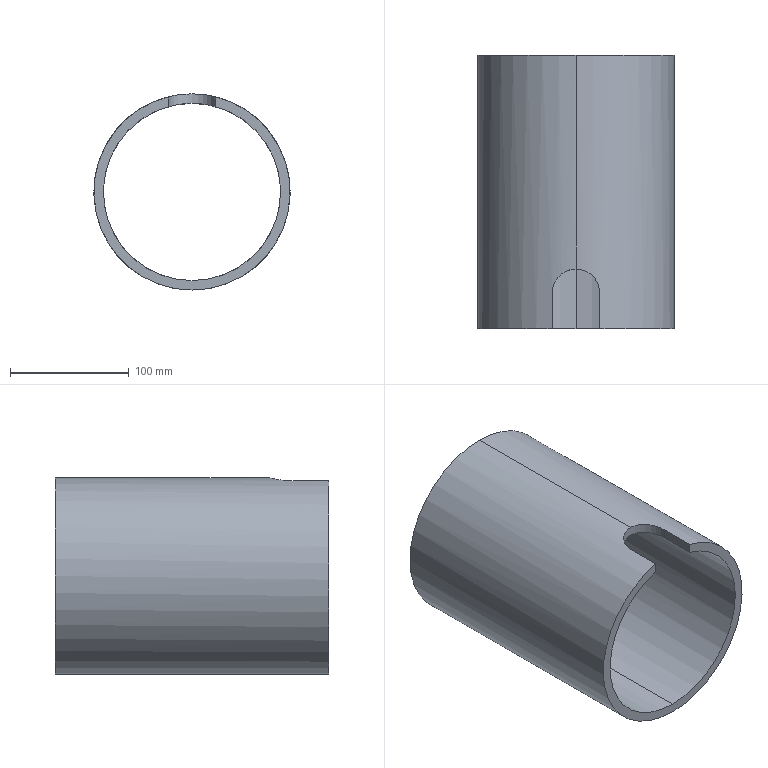Part | SolidWorks | features Extrusion 1, ICE 1 | 1 solid | 9 faces | box 165 x 230 x 165 mm | volume 892768 mm3 | cylinder 5 | plane 4 | commonest cylinder face diameters 149 x2 165 x2 40 x1
STEP:
#1=CARTESIAN_POINT('',(0.,230.,-74.5));
#2=VERTEX_POINT('',#1);
#3=CARTESIAN_POINT('',(0.,230.,74.5));
#4=VERTEX_POINT('',#3);
#5=CARTESIAN_POINT('',(0.,230.,0.));
#6=DIRECTION('',(0.,1.,0.));
#7=DIRECTION('',(0.,0.,1.));
#8=AXIS2_PLACEMENT_3D('',#5,#6,#7);
#9=CIRCLE('',#8,74.5);
#10=EDGE_CURVE('',#2,#4,#9,.T.);
#11=ORIENTED_EDGE('',*,*,#10,.T.);
#12=CARTESIAN_POINT('',(0.,50.,74.5));
#13=VERTEX_POINT('',#12);
#14=CARTESIAN_POINT('',(0.,230.,74.5));
#15=DIRECTION('',(0.,-1.,0.));
#16=VECTOR('',#15,1000.);
#17=LINE('',#14,#16);
#18=EDGE_CURVE('',#4,#13,#17,.T.);
#19=ORIENTED_EDGE('',*,*,#18,.T.);
#20=CARTESIAN_POINT('',(-20.,30.,71.765));
#21=VERTEX_POINT('',#20);
#22=CARTESIAN_POINT('',(-20.,30.,71.765));
#23=CARTESIAN_POINT('',(-20.,31.328,71.765));
#24=CARTESIAN_POINT('',(-19.869,32.633,71.802));
#25=CARTESIAN_POINT('',(-19.485,34.557,71.907));
#26=CARTESIAN_POINT('',(-19.325,35.193,71.95));
#27=CARTESIAN_POINT('',(-18.942,36.453,72.052));
#28=CARTESIAN_POINT('',(-18.717,37.077,72.111));
#29=CARTESIAN_POINT('',(-17.962,38.892,72.304));
#30=CARTESIAN_POINT('',(-17.347,40.038,72.456));
#31=CARTESIAN_POINT('',(-16.258,41.666,72.705));
#32=CARTESIAN_POINT('',(-15.865,42.195,72.792));
#33=CARTESIAN_POINT('',(-15.033,43.207,72.969));
#34=CARTESIAN_POINT('',(-14.595,43.689,73.058));
#35=CARTESIAN_POINT('',(-13.218,45.066,73.324));
#36=CARTESIAN_POINT('',(-12.214,45.892,73.5));
#37=CARTESIAN_POINT('',(-10.575,46.989,73.748));
#38=CARTESIAN_POINT('',(-10.011,47.327,73.827));
#39=CARTESIAN_POINT('',(-8.86,47.942,73.974));
#40=CARTESIAN_POINT('',(-8.272,48.221,74.042));
#41=CARTESIAN_POINT('',(-7.069,48.72,74.166));
#42=CARTESIAN_POINT('',(-6.455,48.941,74.223));
#43=CARTESIAN_POINT('',(-5.199,49.324,74.321));
#44=CARTESIAN_POINT('',(-4.553,49.486,74.364));
#45=CARTESIAN_POINT('',(-2.614,49.872,74.465));
#46=CARTESIAN_POINT('',(-1.312,50.,74.5));
#47=CARTESIAN_POINT('',(0.,50.,74.5));
#48=B_SPLINE_CURVE_WITH_KNOTS('',3,(#22,#23,#24,#25,#26,#27,#28,#29,#30,#31,#32,#33,#34,#35,#36,#37,#38,#39,#40,#41,#42,#43,#44,#45,#46,#47),.UNSPECIFIED.,.F.,.F.,(4,2,2,2,2,2,2,2,2,2,2,2,4),(0.,0.003927,0.005891,0.007854,0.01178,0.01375,0.01571,0.01964,0.0216,0.02356,0.02553,0.02749,0.03142),.UNSPECIFIED.);
#49=EDGE_CURVE('',#21,#13,#48,.T.);
#50=ORIENTED_EDGE('',*,*,#49,.F.);
#51=CARTESIAN_POINT('',(-20.,0.,71.765));
#52=VERTEX_POINT('',#51);
#53=CARTESIAN_POINT('',(-20.,230.,71.765));
#54=DIRECTION('',(0.,1.,0.));
#55=VECTOR('',#54,1000.);
#56=LINE('',#53,#55);
#57=EDGE_CURVE('',#52,#21,#56,.T.);
#58=ORIENTED_EDGE('',*,*,#57,.F.);
#59=CARTESIAN_POINT('',(0.,0.,-74.5));
#60=VERTEX_POINT('',#59);
#61=CARTESIAN_POINT('',(0.,0.,0.));
#62=DIRECTION('',(0.,1.,0.));
#63=DIRECTION('',(0.,0.,1.));
#64=AXIS2_PLACEMENT_3D('',#61,#62,#63);
#65=CIRCLE('',#64,74.5);
#66=EDGE_CURVE('',#60,#52,#65,.T.);
#67=ORIENTED_EDGE('',*,*,#66,.F.);
#68=CARTESIAN_POINT('',(0.,230.,-74.5));
#69=DIRECTION('',(0.,-1.,0.));
#70=VECTOR('',#69,1000.);
#71=LINE('',#68,#70);
#72=EDGE_CURVE('',#2,#60,#71,.T.);
#73=ORIENTED_EDGE('',*,*,#72,.F.);
#74=EDGE_LOOP('',(#11,#19,#50,#58,#67,#73));
#75=FACE_OUTER_BOUND('',#74,.T.);
#76=CARTESIAN_POINT('',(0.,230.,0.));
#77=DIRECTION('',(0.,-1.,0.));
#78=DIRECTION('',(0.,0.,-1.));
#79=AXIS2_PLACEMENT_3D('',#76,#77,#78);
#80=CYLINDRICAL_SURFACE('',#79,74.5);
#81=ADVANCED_FACE('',(#75),#80,.F.);
#82=CARTESIAN_POINT('',(0.,230.,82.5));
#83=VERTEX_POINT('',#82);
#84=CARTESIAN_POINT('',(0.,230.,-82.5));
#85=VERTEX_POINT('',#84);
#86=CARTESIAN_POINT('',(0.,230.,0.));
#87=DIRECTION('',(0.,1.,0.));
#88=DIRECTION('',(0.,0.,1.));
#89=AXIS2_PLACEMENT_3D('',#86,#87,#88);
#90=CIRCLE('',#89,82.5);
#91=EDGE_CURVE('',#83,#85,#90,.T.);
#92=ORIENTED_EDGE('',*,*,#91,.F.);
#93=CARTESIAN_POINT('',(0.,50.,82.5));
#94=VERTEX_POINT('',#93);
#95=CARTESIAN_POINT('',(0.,230.,82.5));
#96=DIRECTION('',(0.,-1.,0.));
#97=VECTOR('',#96,1000.);
#98=LINE('',#95,#97);
#99=EDGE_CURVE('',#83,#94,#98,.T.);
#100=ORIENTED_EDGE('',*,*,#99,.T.);
#101=CARTESIAN_POINT('',(20.,30.,80.039));
#102=VERTEX_POINT('',#101);
#103=CARTESIAN_POINT('',(0.,50.,82.5));
#104=CARTESIAN_POINT('',(0.6545,50.,82.5));
#105=CARTESIAN_POINT('',(1.311,49.968,82.492));
#106=CARTESIAN_POINT('',(2.629,49.837,82.461));
#107=CARTESIAN_POINT('',(3.281,49.74,82.437));
#108=CARTESIAN_POINT('',(5.206,49.355,82.346));
#109=CARTESIAN_POINT('',(6.454,48.976,82.256));
#110=CARTESIAN_POINT('',(8.273,48.22,82.086));
#111=CARTESIAN_POINT('',(8.871,47.937,82.024));
#112=CARTESIAN_POINT('',(10.024,47.319,81.891));
#113=CARTESIAN_POINT('',(10.581,46.984,81.82));
#114=CARTESIAN_POINT('',(11.661,46.262,81.674));
#115=CARTESIAN_POINT('',(12.183,45.874,81.597));
#116=CARTESIAN_POINT('',(12.939,45.254,81.479));
#117=CARTESIAN_POINT('',(13.186,45.041,81.44));
#118=CARTESIAN_POINT('',(13.672,44.601,81.36));
#119=CARTESIAN_POINT('',(13.911,44.374,81.319));
#120=CARTESIAN_POINT('',(15.068,43.216,81.118));
#121=CARTESIAN_POINT('',(15.892,42.212,80.958));
#122=CARTESIAN_POINT('',(16.977,40.593,80.735));
#123=CARTESIAN_POINT('',(17.314,40.033,80.663));
#124=CARTESIAN_POINT('',(17.935,38.875,80.528));
#125=CARTESIAN_POINT('',(18.217,38.28,80.464));
#126=CARTESIAN_POINT('',(18.969,36.47,80.291));
#127=CARTESIAN_POINT('',(19.35,35.225,80.199));
#128=CARTESIAN_POINT('',(19.737,33.296,80.104));
#129=CARTESIAN_POINT('',(19.836,32.64,80.08));
#130=CARTESIAN_POINT('',(19.967,31.323,80.047));
#131=CARTESIAN_POINT('',(20.,30.663,80.039));
#132=CARTESIAN_POINT('',(20.,30.,80.039));
#133=B_SPLINE_CURVE_WITH_KNOTS('',3,(#103,#104,#105,#106,#107,#108,#109,#110,#111,#112,#113,#114,#115,#116,#117,#118,#119,#120,#121,#122,#123,#124,#125,#126,#127,#128,#129,#130,#131,#132),.UNSPECIFIED.,.F.,.F.,(4,2,2,2,2,2,2,2,2,2,2,2,2,2,4),(0.03139,0.03335,0.03531,0.03923,0.04119,0.04315,0.04511,0.04609,0.04707,0.05099,0.05295,0.05491,0.05883,0.06078,0.06274),.UNSPECIFIED.);
#134=EDGE_CURVE('',#94,#102,#133,.T.);
#135=ORIENTED_EDGE('',*,*,#134,.T.);
#136=CARTESIAN_POINT('',(20.,0.,80.039));
#137=VERTEX_POINT('',#136);
#138=CARTESIAN_POINT('',(20.,230.,80.039));
#139=DIRECTION('',(0.,-1.,0.));
#140=VECTOR('',#139,1000.);
#141=LINE('',#138,#140);
#142=EDGE_CURVE('',#102,#137,#141,.T.);
#143=ORIENTED_EDGE('',*,*,#142,.T.);
#144=CARTESIAN_POINT('',(0.,0.,-82.5));
#145=VERTEX_POINT('',#144);
#146=CARTESIAN_POINT('',(0.,0.,0.));
#147=DIRECTION('',(0.,1.,0.));
#148=DIRECTION('',(0.,0.,1.));
#149=AXIS2_PLACEMENT_3D('',#146,#147,#148);
#150=CIRCLE('',#149,82.5);
#151=EDGE_CURVE('',#137,#145,#150,.T.);
#152=ORIENTED_EDGE('',*,*,#151,.T.);
#153=CARTESIAN_POINT('',(0.,230.,-82.5));
#154=DIRECTION('',(0.,-1.,0.));
#155=VECTOR('',#154,1000.);
#156=LINE('',#153,#155);
#157=EDGE_CURVE('',#85,#145,#156,.T.);
#158=ORIENTED_EDGE('',*,*,#157,.F.);
#159=EDGE_LOOP('',(#92,#100,#135,#143,#152,#158));
#160=FACE_OUTER_BOUND('',#159,.T.);
#161=CARTESIAN_POINT('',(0.,230.,0.));
#162=DIRECTION('',(0.,-1.,0.));
#163=DIRECTION('',(0.,0.,-1.));
#164=AXIS2_PLACEMENT_3D('',#161,#162,#163);
#165=CYLINDRICAL_SURFACE('',#164,82.5);
#166=ADVANCED_FACE('',(#160),#165,.T.);
#167=CARTESIAN_POINT('',(20.,0.,71.765));
#168=VERTEX_POINT('',#167);
#169=CARTESIAN_POINT('',(20.,0.,82.501));
#170=DIRECTION('',(0.,0.,-1.));
#171=VECTOR('',#170,1000.);
#172=LINE('',#169,#171);
#173=EDGE_CURVE('',#137,#168,#172,.T.);
#174=ORIENTED_EDGE('',*,*,#173,.T.);
#175=CARTESIAN_POINT('',(0.,0.,0.));
#176=DIRECTION('',(0.,1.,0.));
#177=DIRECTION('',(0.,0.,1.));
#178=AXIS2_PLACEMENT_3D('',#175,#176,#177);
#179=CIRCLE('',#178,74.5);
#180=EDGE_CURVE('',#168,#60,#179,.T.);
#181=ORIENTED_EDGE('',*,*,#180,.T.);
#182=ORIENTED_EDGE('',*,*,#66,.T.);
#183=CARTESIAN_POINT('',(-20.,0.,80.039));
#184=VERTEX_POINT('',#183);
#185=CARTESIAN_POINT('',(-20.,0.,82.501));
#186=DIRECTION('',(0.,0.,-1.));
#187=VECTOR('',#186,1000.);
#188=LINE('',#185,#187);
#189=EDGE_CURVE('',#184,#52,#188,.T.);
#190=ORIENTED_EDGE('',*,*,#189,.F.);
#191=CARTESIAN_POINT('',(0.,0.,0.));
#192=DIRECTION('',(0.,1.,0.));
#193=DIRECTION('',(0.,0.,1.));
#194=AXIS2_PLACEMENT_3D('',#191,#192,#193);
#195=CIRCLE('',#194,82.5);
#196=EDGE_CURVE('',#145,#184,#195,.T.);
#197=ORIENTED_EDGE('',*,*,#196,.F.);
#198=ORIENTED_EDGE('',*,*,#151,.F.);
#199=EDGE_LOOP('',(#174,#181,#182,#190,#197,#198));
#200=FACE_OUTER_BOUND('',#199,.T.);
#201=CARTESIAN_POINT('',(0.,0.,0.));
#202=DIRECTION('',(0.,1.,0.));
#203=DIRECTION('',(0.,0.,1.));
#204=AXIS2_PLACEMENT_3D('',#201,#202,#203);
#205=PLANE('',#204);
#206=ADVANCED_FACE('',(#200),#205,.F.);
#207=ORIENTED_EDGE('',*,*,#99,.F.);
#208=CARTESIAN_POINT('',(0.,230.,0.));
#209=DIRECTION('',(0.,1.,0.));
#210=DIRECTION('',(0.,0.,1.));
#211=AXIS2_PLACEMENT_3D('',#208,#209,#210);
#212=CIRCLE('',#211,82.5);
#213=EDGE_CURVE('',#85,#83,#212,.T.);
#214=ORIENTED_EDGE('',*,*,#213,.F.);
#215=ORIENTED_EDGE('',*,*,#157,.T.);
#216=ORIENTED_EDGE('',*,*,#196,.T.);
#217=CARTESIAN_POINT('',(-20.,30.,80.039));
#218=VERTEX_POINT('',#217);
#219=CARTESIAN_POINT('',(-20.,230.,80.039));
#220=DIRECTION('',(0.,1.,0.));
#221=VECTOR('',#220,1000.);
#222=LINE('',#219,#221);
#223=EDGE_CURVE('',#184,#218,#222,.T.);
#224=ORIENTED_EDGE('',*,*,#223,.T.);
#225=CARTESIAN_POINT('',(-20.,30.,80.039));
#226=CARTESIAN_POINT('',(-20.,31.327,80.039));
#227=CARTESIAN_POINT('',(-19.869,32.631,80.072));
#228=CARTESIAN_POINT('',(-19.486,34.554,80.166));
#229=CARTESIAN_POINT('',(-19.326,35.189,80.205));
#230=CARTESIAN_POINT('',(-18.943,36.449,80.296));
#231=CARTESIAN_POINT('',(-18.719,37.073,80.349));
#232=CARTESIAN_POINT('',(-17.964,38.888,80.522));
#233=CARTESIAN_POINT('',(-17.349,40.035,80.659));
#234=CARTESIAN_POINT('',(-16.442,41.392,80.845));
#235=CARTESIAN_POINT('',(-16.253,41.659,80.883));
#236=CARTESIAN_POINT('',(-15.862,42.186,80.961));
#237=CARTESIAN_POINT('',(-15.659,42.446,81.001));
#238=CARTESIAN_POINT('',(-15.034,43.206,81.12));
#239=CARTESIAN_POINT('',(-14.596,43.689,81.2));
#240=CARTESIAN_POINT('',(-13.217,45.067,81.44));
#241=CARTESIAN_POINT('',(-12.212,45.893,81.599));
#242=CARTESIAN_POINT('',(-10.573,46.99,81.822));
#243=CARTESIAN_POINT('',(-10.008,47.328,81.893));
#244=CARTESIAN_POINT('',(-8.857,47.944,82.025));
#245=CARTESIAN_POINT('',(-8.268,48.223,82.087));
#246=CARTESIAN_POINT('',(-7.065,48.722,82.199));
#247=CARTESIAN_POINT('',(-6.451,48.942,82.25));
#248=CARTESIAN_POINT('',(-5.195,49.325,82.339));
#249=CARTESIAN_POINT('',(-4.551,49.487,82.377));
#250=CARTESIAN_POINT('',(-2.612,49.872,82.469));
#251=CARTESIAN_POINT('',(-1.31,50.,82.5));
#252=CARTESIAN_POINT('',(0.,50.,82.5));
#253=B_SPLINE_CURVE_WITH_KNOTS('',3,(#225,#226,#227,#228,#229,#230,#231,#232,#233,#234,#235,#236,#237,#238,#239,#240,#241,#242,#243,#244,#245,#246,#247,#248,#249,#250,#251,#252),.UNSPECIFIED.,.F.,.F.,(4,2,2,2,2,2,2,2,2,2,2,2,2,4),(0.,0.003924,0.005886,0.007847,0.01177,0.01275,0.01373,0.01569,0.01962,0.02158,0.02354,0.0255,0.02747,0.03139),.UNSPECIFIED.);
#254=EDGE_CURVE('',#218,#94,#253,.T.);
#255=ORIENTED_EDGE('',*,*,#254,.T.);
#256=EDGE_LOOP('',(#207,#214,#215,#216,#224,#255));
#257=FACE_OUTER_BOUND('',#256,.T.);
#258=CARTESIAN_POINT('',(0.,230.,0.));
#259=DIRECTION('',(0.,-1.,0.));
#260=DIRECTION('',(0.,0.,-1.));
#261=AXIS2_PLACEMENT_3D('',#258,#259,#260);
#262=CYLINDRICAL_SURFACE('',#261,82.5);
#263=ADVANCED_FACE('',(#257),#262,.T.);
#264=ORIENTED_EDGE('',*,*,#18,.F.);
#265=CARTESIAN_POINT('',(0.,230.,0.));
#266=DIRECTION('',(0.,1.,0.));
#267=DIRECTION('',(0.,0.,1.));
#268=AXIS2_PLACEMENT_3D('',#265,#266,#267);
#269=CIRCLE('',#268,74.5);
#270=EDGE_CURVE('',#4,#2,#269,.T.);
#271=ORIENTED_EDGE('',*,*,#270,.T.);
#272=ORIENTED_EDGE('',*,*,#72,.T.);
#273=ORIENTED_EDGE('',*,*,#180,.F.);
#274=CARTESIAN_POINT('',(20.,30.,71.765));
#275=VERTEX_POINT('',#274);
#276=CARTESIAN_POINT('',(20.,230.,71.765));
#277=DIRECTION('',(0.,-1.,0.));
#278=VECTOR('',#277,1000.);
#279=LINE('',#276,#278);
#280=EDGE_CURVE('',#275,#168,#279,.T.);
#281=ORIENTED_EDGE('',*,*,#280,.F.);
#282=CARTESIAN_POINT('',(0.,50.,74.5));
#283=CARTESIAN_POINT('',(0.6551,50.,74.5));
#284=CARTESIAN_POINT('',(1.313,49.968,74.491));
#285=CARTESIAN_POINT('',(2.632,49.837,74.456));
#286=CARTESIAN_POINT('',(3.283,49.74,74.43));
#287=CARTESIAN_POINT('',(5.209,49.354,74.329));
#288=CARTESIAN_POINT('',(6.458,48.974,74.23));
#289=CARTESIAN_POINT('',(8.278,48.218,74.041));
#290=CARTESIAN_POINT('',(8.876,47.935,73.972));
#291=CARTESIAN_POINT('',(10.027,47.317,73.824));
#292=CARTESIAN_POINT('',(10.584,46.982,73.746));
#293=CARTESIAN_POINT('',(11.664,46.26,73.583));
#294=CARTESIAN_POINT('',(12.185,45.873,73.499));
#295=CARTESIAN_POINT('',(13.193,45.046,73.324));
#296=CARTESIAN_POINT('',(13.681,44.603,73.235));
#297=CARTESIAN_POINT('',(15.068,43.217,72.966));
#298=CARTESIAN_POINT('',(15.89,42.214,72.789));
#299=CARTESIAN_POINT('',(16.975,40.595,72.541));
#300=CARTESIAN_POINT('',(17.312,40.036,72.461));
#301=CARTESIAN_POINT('',(17.934,38.877,72.31));
#302=CARTESIAN_POINT('',(18.216,38.283,72.239));
#303=CARTESIAN_POINT('',(18.968,36.475,72.047));
#304=CARTESIAN_POINT('',(19.349,35.23,71.944));
#305=CARTESIAN_POINT('',(19.737,33.298,71.838));
#306=CARTESIAN_POINT('',(19.836,32.641,71.811));
#307=CARTESIAN_POINT('',(19.967,31.324,71.774));
#308=CARTESIAN_POINT('',(20.,30.663,71.765));
#309=CARTESIAN_POINT('',(20.,30.,71.765));
#310=B_SPLINE_CURVE_WITH_KNOTS('',3,(#282,#283,#284,#285,#286,#287,#288,#289,#290,#291,#292,#293,#294,#295,#296,#297,#298,#299,#300,#301,#302,#303,#304,#305,#306,#307,#308,#309),.UNSPECIFIED.,.F.,.F.,(4,2,2,2,2,2,2,2,2,2,2,2,2,4),(0.03142,0.03338,0.03534,0.03926,0.04122,0.04318,0.04515,0.04711,0.05103,0.05299,0.05495,0.05888,0.06084,0.0628),.UNSPECIFIED.);
#311=EDGE_CURVE('',#13,#275,#310,.T.);
#312=ORIENTED_EDGE('',*,*,#311,.F.);
#313=EDGE_LOOP('',(#264,#271,#272,#273,#281,#312));
#314=FACE_OUTER_BOUND('',#313,.T.);
#315=CARTESIAN_POINT('',(0.,230.,0.));
#316=DIRECTION('',(0.,-1.,0.));
#317=DIRECTION('',(0.,0.,-1.));
#318=AXIS2_PLACEMENT_3D('',#315,#316,#317);
#319=CYLINDRICAL_SURFACE('',#318,74.5);
#320=ADVANCED_FACE('',(#314),#319,.F.);
#321=ORIENTED_EDGE('',*,*,#213,.T.);
#322=ORIENTED_EDGE('',*,*,#91,.T.);
#323=EDGE_LOOP('',(#321,#322));
#324=FACE_OUTER_BOUND('',#323,.T.);
#325=ORIENTED_EDGE('',*,*,#10,.F.);
#326=ORIENTED_EDGE('',*,*,#270,.F.);
#327=EDGE_LOOP('',(#325,#326));
#328=FACE_BOUND('',#327,.T.);
#329=CARTESIAN_POINT('',(0.,230.,0.));
#330=DIRECTION('',(0.,1.,0.));
#331=DIRECTION('',(0.,0.,1.));
#332=AXIS2_PLACEMENT_3D('',#329,#330,#331);
#333=PLANE('',#332);
#334=ADVANCED_FACE('',(#324,#328),#333,.T.);
#335=CARTESIAN_POINT('',(20.,30.,82.501));
#336=DIRECTION('',(0.,0.,-1.));
#337=VECTOR('',#336,1000.);
#338=LINE('',#335,#337);
#339=EDGE_CURVE('',#102,#275,#338,.T.);
#340=ORIENTED_EDGE('',*,*,#339,.T.);
#341=ORIENTED_EDGE('',*,*,#280,.T.);
#342=ORIENTED_EDGE('',*,*,#173,.F.);
#343=ORIENTED_EDGE('',*,*,#142,.F.);
#344=EDGE_LOOP('',(#340,#341,#342,#343));
#345=FACE_OUTER_BOUND('',#344,.T.);
#346=CARTESIAN_POINT('',(20.,0.,82.501));
#347=DIRECTION('',(-1.,0.,0.));
#348=DIRECTION('',(0.,-1.,0.));
#349=AXIS2_PLACEMENT_3D('',#346,#347,#348);
#350=PLANE('',#349);
#351=ADVANCED_FACE('',(#345),#350,.T.);
#352=CARTESIAN_POINT('',(-20.,30.,82.501));
#353=DIRECTION('',(0.,0.,-1.));
#354=VECTOR('',#353,1000.);
#355=LINE('',#352,#354);
#356=EDGE_CURVE('',#218,#21,#355,.T.);
#357=ORIENTED_EDGE('',*,*,#356,.T.);
#358=ORIENTED_EDGE('',*,*,#49,.T.);
#359=ORIENTED_EDGE('',*,*,#311,.T.);
#360=ORIENTED_EDGE('',*,*,#339,.F.);
#361=ORIENTED_EDGE('',*,*,#134,.F.);
#362=ORIENTED_EDGE('',*,*,#254,.F.);
#363=EDGE_LOOP('',(#357,#358,#359,#360,#361,#362));
#364=FACE_OUTER_BOUND('',#363,.T.);
#365=CARTESIAN_POINT('',(0.,30.,82.501));
#366=DIRECTION('',(0.,0.,-1.));
#367=DIRECTION('',(-1.,0.,0.));
#368=AXIS2_PLACEMENT_3D('',#365,#366,#367);
#369=CYLINDRICAL_SURFACE('',#368,20.);
#370=ADVANCED_FACE('',(#364),#369,.F.);
#371=ORIENTED_EDGE('',*,*,#189,.T.);
#372=ORIENTED_EDGE('',*,*,#57,.T.);
#373=ORIENTED_EDGE('',*,*,#356,.F.);
#374=ORIENTED_EDGE('',*,*,#223,.F.);
#375=EDGE_LOOP('',(#371,#372,#373,#374));
#376=FACE_OUTER_BOUND('',#375,.T.);
#377=CARTESIAN_POINT('',(-20.,0.,82.501));
#378=DIRECTION('',(1.,0.,0.));
#379=DIRECTION('',(0.,0.,-1.));
#380=AXIS2_PLACEMENT_3D('',#377,#378,#379);
#381=PLANE('',#380);
#382=ADVANCED_FACE('',(#376),#381,.T.);
#383=CLOSED_SHELL('',(#81,#166,#206,#263,#320,#334,#351,#370,#382));
#384=MANIFOLD_SOLID_BREP('',#383);
#385=CARTESIAN_POINT('',(0.,0.,0.));
#386=DIRECTION('',(0.,0.,1.));
#387=DIRECTION('',(1.,0.,0.));
#388=AXIS2_PLACEMENT_3D('',#385,#386,#387);
#389=(LENGTH_UNIT()NAMED_UNIT(*)SI_UNIT(.MILLI.,.METRE.));
#390=UNCERTAINTY_MEASURE_WITH_UNIT(LENGTH_MEASURE(0.00001),#389,'','');
#391=(NAMED_UNIT(*)PLANE_ANGLE_UNIT()SI_UNIT($,.RADIAN.));
#392=(NAMED_UNIT(*)SI_UNIT($,.STERADIAN.)SOLID_ANGLE_UNIT());
#393=(GEOMETRIC_REPRESENTATION_CONTEXT(3)GLOBAL_UNCERTAINTY_ASSIGNED_CONTEXT((#390))GLOBAL_UNIT_ASSIGNED_CONTEXT((#389,#391,#392))REPRESENTATION_CONTEXT('',''));
#394=ADVANCED_BREP_SHAPE_REPRESENTATION('',(#384,#388),#393);